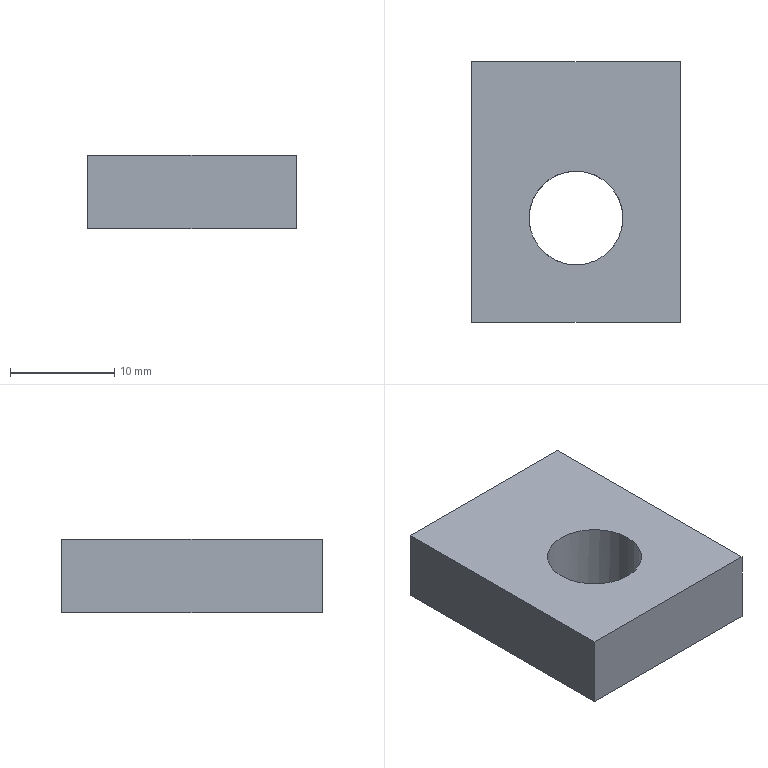Part | STEP file | 1 solid | 7 faces | box 20 x 25 x 7 mm | volume 3055 mm3 | plane 6 | cylinder 1 | commonest cylinder face diameters 9 x1
STEP:
#1=CARTESIAN_POINT('',(-254.,-155.96,-50.));
#2=VERTEX_POINT('',#1);
#3=CARTESIAN_POINT('',(-254.,-180.96,-50.));
#4=VERTEX_POINT('',#3);
#5=CARTESIAN_POINT('',(-254.,-155.96,-50.));
#6=DIRECTION('',(0.,-1.,0.));
#7=VECTOR('',#6,1.);
#8=LINE('',#5,#7);
#9=EDGE_CURVE('',#2,#4,#8,.T.);
#10=ORIENTED_EDGE('',*,*,#9,.T.);
#11=CARTESIAN_POINT('',(-254.,-180.96,-43.));
#12=VERTEX_POINT('',#11);
#13=CARTESIAN_POINT('',(-254.,-180.96,-43.));
#14=DIRECTION('',(0.,0.,-1.));
#15=VECTOR('',#14,1.);
#16=LINE('',#13,#15);
#17=EDGE_CURVE('',#12,#4,#16,.T.);
#18=ORIENTED_EDGE('',*,*,#17,.F.);
#19=CARTESIAN_POINT('',(-254.,-155.96,-43.));
#20=VERTEX_POINT('',#19);
#21=CARTESIAN_POINT('',(-254.,-155.96,-43.));
#22=DIRECTION('',(0.,-1.,0.));
#23=VECTOR('',#22,1.);
#24=LINE('',#21,#23);
#25=EDGE_CURVE('',#20,#12,#24,.T.);
#26=ORIENTED_EDGE('',*,*,#25,.F.);
#27=CARTESIAN_POINT('',(-254.,-155.96,-43.));
#28=DIRECTION('',(0.,0.,-1.));
#29=VECTOR('',#28,1.);
#30=LINE('',#27,#29);
#31=EDGE_CURVE('',#20,#2,#30,.T.);
#32=ORIENTED_EDGE('',*,*,#31,.T.);
#33=EDGE_LOOP('',(#10,#18,#26,#32));
#34=FACE_OUTER_BOUND('',#33,.T.);
#35=CARTESIAN_POINT('',(-254.,-155.96,-43.));
#36=DIRECTION('',(1.,0.,0.));
#37=DIRECTION('',(0.,0.,-1.));
#38=AXIS2_PLACEMENT_3D('',#35,#36,#37);
#39=PLANE('',#38);
#40=ADVANCED_FACE('',(#34),#39,.F.);
#41=CARTESIAN_POINT('',(-234.,-180.96,-50.));
#42=VERTEX_POINT('',#41);
#43=CARTESIAN_POINT('',(-254.,-180.96,-50.));
#44=DIRECTION('',(1.,0.,0.));
#45=VECTOR('',#44,1.);
#46=LINE('',#43,#45);
#47=EDGE_CURVE('',#4,#42,#46,.T.);
#48=ORIENTED_EDGE('',*,*,#47,.T.);
#49=CARTESIAN_POINT('',(-234.,-180.96,-43.));
#50=VERTEX_POINT('',#49);
#51=CARTESIAN_POINT('',(-234.,-180.96,-43.));
#52=DIRECTION('',(0.,0.,-1.));
#53=VECTOR('',#52,1.);
#54=LINE('',#51,#53);
#55=EDGE_CURVE('',#50,#42,#54,.T.);
#56=ORIENTED_EDGE('',*,*,#55,.F.);
#57=CARTESIAN_POINT('',(-254.,-180.96,-43.));
#58=DIRECTION('',(1.,0.,0.));
#59=VECTOR('',#58,1.);
#60=LINE('',#57,#59);
#61=EDGE_CURVE('',#12,#50,#60,.T.);
#62=ORIENTED_EDGE('',*,*,#61,.F.);
#63=ORIENTED_EDGE('',*,*,#17,.T.);
#64=EDGE_LOOP('',(#48,#56,#62,#63));
#65=FACE_OUTER_BOUND('',#64,.T.);
#66=CARTESIAN_POINT('',(-254.,-180.96,-43.));
#67=DIRECTION('',(0.,1.,0.));
#68=DIRECTION('',(0.,0.,1.));
#69=AXIS2_PLACEMENT_3D('',#66,#67,#68);
#70=PLANE('',#69);
#71=ADVANCED_FACE('',(#65),#70,.F.);
#72=CARTESIAN_POINT('',(-234.,-155.96,-50.));
#73=VERTEX_POINT('',#72);
#74=CARTESIAN_POINT('',(-234.,-180.96,-50.));
#75=DIRECTION('',(0.,1.,0.));
#76=VECTOR('',#75,1.);
#77=LINE('',#74,#76);
#78=EDGE_CURVE('',#42,#73,#77,.T.);
#79=ORIENTED_EDGE('',*,*,#78,.T.);
#80=CARTESIAN_POINT('',(-234.,-155.96,-43.));
#81=VERTEX_POINT('',#80);
#82=CARTESIAN_POINT('',(-234.,-155.96,-43.));
#83=DIRECTION('',(0.,0.,-1.));
#84=VECTOR('',#83,1.);
#85=LINE('',#82,#84);
#86=EDGE_CURVE('',#81,#73,#85,.T.);
#87=ORIENTED_EDGE('',*,*,#86,.F.);
#88=CARTESIAN_POINT('',(-234.,-180.96,-43.));
#89=DIRECTION('',(0.,1.,0.));
#90=VECTOR('',#89,1.);
#91=LINE('',#88,#90);
#92=EDGE_CURVE('',#50,#81,#91,.T.);
#93=ORIENTED_EDGE('',*,*,#92,.F.);
#94=ORIENTED_EDGE('',*,*,#55,.T.);
#95=EDGE_LOOP('',(#79,#87,#93,#94));
#96=FACE_OUTER_BOUND('',#95,.T.);
#97=CARTESIAN_POINT('',(-234.,-180.96,-43.));
#98=DIRECTION('',(-1.,0.,0.));
#99=DIRECTION('',(0.,0.,1.));
#100=AXIS2_PLACEMENT_3D('',#97,#98,#99);
#101=PLANE('',#100);
#102=ADVANCED_FACE('',(#96),#101,.F.);
#103=CARTESIAN_POINT('',(-234.,-155.96,-50.));
#104=DIRECTION('',(-1.,0.,0.));
#105=VECTOR('',#104,1.);
#106=LINE('',#103,#105);
#107=EDGE_CURVE('',#73,#2,#106,.T.);
#108=ORIENTED_EDGE('',*,*,#107,.T.);
#109=ORIENTED_EDGE('',*,*,#31,.F.);
#110=CARTESIAN_POINT('',(-234.,-155.96,-43.));
#111=DIRECTION('',(-1.,0.,0.));
#112=VECTOR('',#111,1.);
#113=LINE('',#110,#112);
#114=EDGE_CURVE('',#81,#20,#113,.T.);
#115=ORIENTED_EDGE('',*,*,#114,.F.);
#116=ORIENTED_EDGE('',*,*,#86,.T.);
#117=EDGE_LOOP('',(#108,#109,#115,#116));
#118=FACE_OUTER_BOUND('',#117,.T.);
#119=CARTESIAN_POINT('',(-234.,-155.96,-43.));
#120=DIRECTION('',(0.,-1.,0.));
#121=DIRECTION('',(0.,0.,-1.));
#122=AXIS2_PLACEMENT_3D('',#119,#120,#121);
#123=PLANE('',#122);
#124=ADVANCED_FACE('',(#118),#123,.F.);
#125=ORIENTED_EDGE('',*,*,#25,.T.);
#126=ORIENTED_EDGE('',*,*,#61,.T.);
#127=ORIENTED_EDGE('',*,*,#92,.T.);
#128=ORIENTED_EDGE('',*,*,#114,.T.);
#129=EDGE_LOOP('',(#125,#126,#127,#128));
#130=FACE_BOUND('',#129,.T.);
#131=CARTESIAN_POINT('',(-248.5,-170.96,-43.));
#132=VERTEX_POINT('',#131);
#133=CARTESIAN_POINT('',(-244.,-170.96,-43.));
#134=DIRECTION('',(0.,0.,1.));
#135=DIRECTION('',(-1.,0.,0.));
#136=AXIS2_PLACEMENT_3D('',#133,#134,#135);
#137=CIRCLE('',#136,4.5);
#138=EDGE_CURVE('',#132,#132,#137,.T.);
#139=ORIENTED_EDGE('',*,*,#138,.F.);
#140=EDGE_LOOP('',(#139));
#141=FACE_BOUND('',#140,.T.);
#142=CARTESIAN_POINT('',(-1288.786,-131.676,-43.));
#143=DIRECTION('',(0.,0.,1.));
#144=DIRECTION('',(1.,0.,0.));
#145=AXIS2_PLACEMENT_3D('',#142,#143,#144);
#146=PLANE('',#145);
#147=ADVANCED_FACE('',(#130,#141),#146,.T.);
#148=CARTESIAN_POINT('',(-239.5,-170.96,-50.));
#149=VERTEX_POINT('',#148);
#150=CARTESIAN_POINT('',(-244.,-170.96,-50.));
#151=DIRECTION('',(0.,0.,1.));
#152=DIRECTION('',(1.,0.,0.));
#153=AXIS2_PLACEMENT_3D('',#150,#151,#152);
#154=CIRCLE('',#153,4.5);
#155=EDGE_CURVE('',#149,#149,#154,.T.);
#156=ORIENTED_EDGE('',*,*,#155,.T.);
#157=EDGE_LOOP('',(#156));
#158=FACE_BOUND('',#157,.T.);
#159=ORIENTED_EDGE('',*,*,#9,.F.);
#160=ORIENTED_EDGE('',*,*,#107,.F.);
#161=ORIENTED_EDGE('',*,*,#78,.F.);
#162=ORIENTED_EDGE('',*,*,#47,.F.);
#163=EDGE_LOOP('',(#159,#160,#161,#162));
#164=FACE_BOUND('',#163,.T.);
#165=CARTESIAN_POINT('',(-1288.786,-131.676,-50.));
#166=DIRECTION('',(0.,0.,1.));
#167=DIRECTION('',(1.,0.,0.));
#168=AXIS2_PLACEMENT_3D('',#165,#166,#167);
#169=PLANE('',#168);
#170=ADVANCED_FACE('',(#158,#164),#169,.F.);
#171=ORIENTED_EDGE('',*,*,#138,.T.);
#172=EDGE_LOOP('',(#171));
#173=FACE_BOUND('',#172,.T.);
#174=ORIENTED_EDGE('',*,*,#155,.F.);
#175=EDGE_LOOP('',(#174));
#176=FACE_BOUND('',#175,.T.);
#177=CARTESIAN_POINT('',(-244.,-170.96,-50.));
#178=DIRECTION('',(0.,0.,1.));
#179=DIRECTION('',(1.,0.,0.));
#180=AXIS2_PLACEMENT_3D('',#177,#178,#179);
#181=CYLINDRICAL_SURFACE('',#180,4.5);
#182=ADVANCED_FACE('',(#173,#176),#181,.F.);
#183=CLOSED_SHELL('',(#40,#71,#102,#124,#147,#170,#182));
#184=MANIFOLD_SOLID_BREP('',#183);
#185=(LENGTH_UNIT()NAMED_UNIT(*)SI_UNIT(.MILLI.,.METRE.));
#186=UNCERTAINTY_MEASURE_WITH_UNIT(LENGTH_MEASURE(0.00002),#185,'','');
#187=(NAMED_UNIT(*)PLANE_ANGLE_UNIT()SI_UNIT($,.RADIAN.));
#188=PLANE_ANGLE_MEASURE_WITH_UNIT(PLANE_ANGLE_MEASURE(0.01745),#187);
#189=DIMENSIONAL_EXPONENTS(0.,0.,0.,0.,0.,0.,0.);
#190=(CONVERSION_BASED_UNIT('DEGREE',#188)NAMED_UNIT(#189)PLANE_ANGLE_UNIT());
#191=(NAMED_UNIT(*)SI_UNIT($,.STERADIAN.)SOLID_ANGLE_UNIT());
#192=(GEOMETRIC_REPRESENTATION_CONTEXT(3)GLOBAL_UNCERTAINTY_ASSIGNED_CONTEXT((#186))GLOBAL_UNIT_ASSIGNED_CONTEXT((#185,#190,#191))REPRESENTATION_CONTEXT('',''));
#193=ADVANCED_BREP_SHAPE_REPRESENTATION('',(#184),#192);